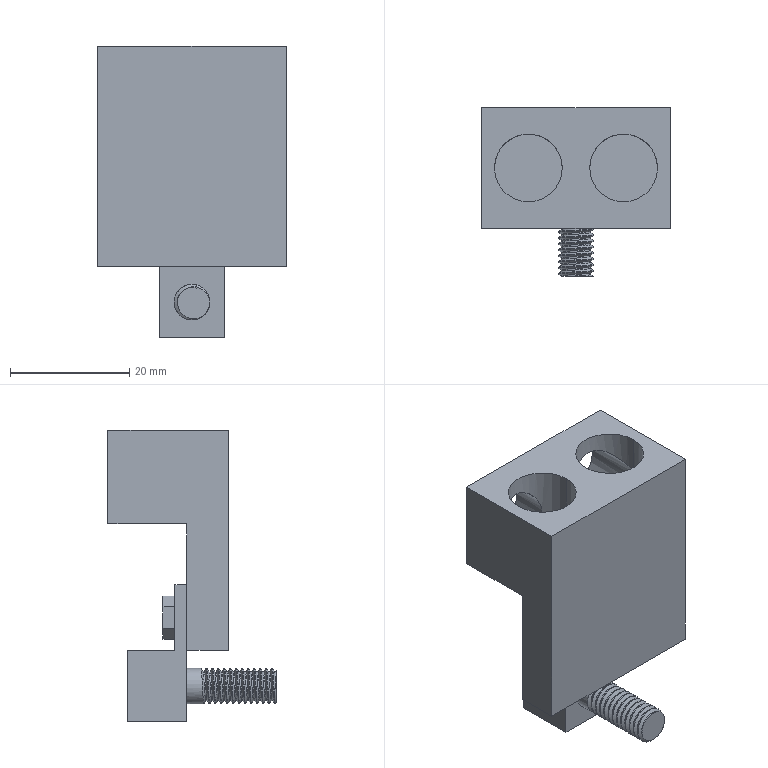Part | SolidWorks | features ICE 8, Extrusion 1, SweepThread 1 | 1 solid | 79 faces | box 31.72 x 28.25 x 48.96 mm | volume 13161 mm3 | plane 40 | cylinder 36 | spline 3 | commonest cylinder face diameters 6 x26 10 x4 11.41 x4 8 x2